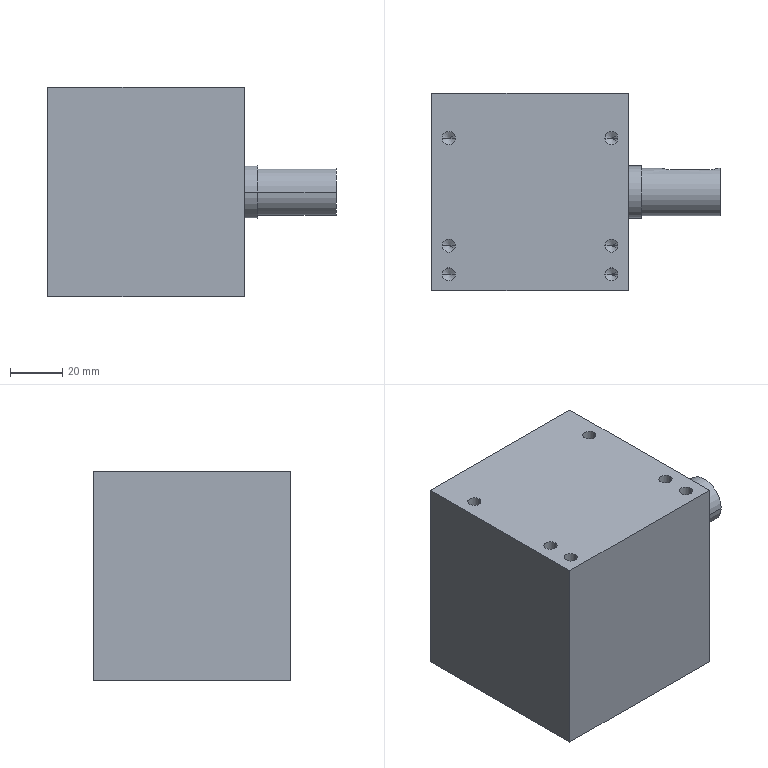Part | SolidWorks | features HoleWzd 3, ICE 3, Extrusion 1 | 1 solid | 61 faces | box 110 x 75 x 80 mm | volume 456028 mm3 | cylinder 28 | cone 22 | plane 11 | commonest cylinder face diameters 5 x14 4.2 x8 6 x2 18 x2 20 x2